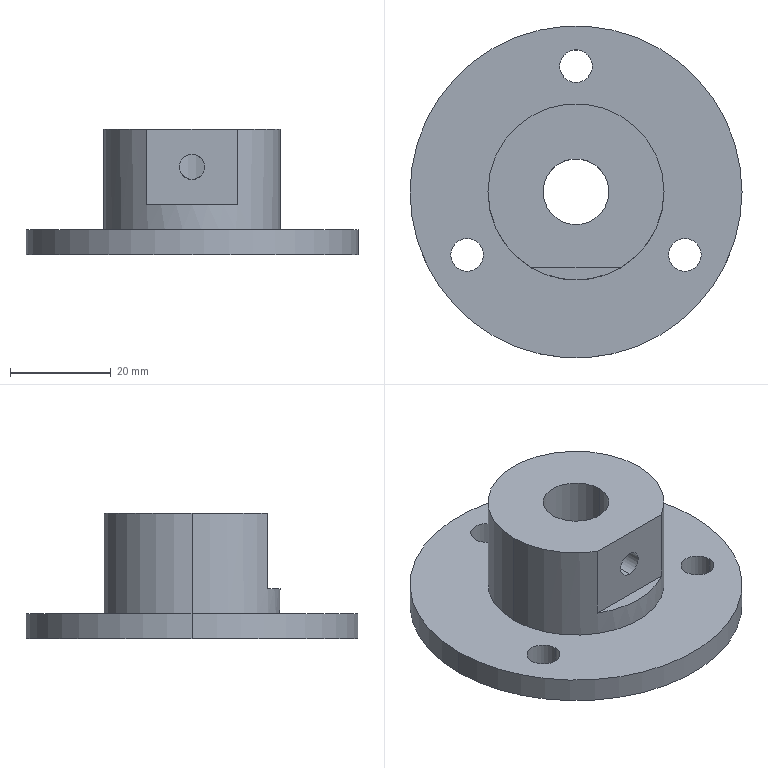Part | STEP file | 11-FG-B05611 | 1 solid | 19 faces | box 66 x 66 x 25 mm | volume 31855 mm3 | cylinder 14 | plane 5 | commonest cylinder face diameters 6.5 x6 5 x2 13.1 x2 35 x2 66 x2
STEP:
#1=CARTESIAN_POINT('',(0.,-6.55,20.));
#2=VERTEX_POINT('',#1);
#3=CARTESIAN_POINT('',(0.,-6.55,15.));
#4=VERTEX_POINT('',#3);
#5=CARTESIAN_POINT('',(0.,-6.55,20.));
#6=CARTESIAN_POINT('',(-0.1643,-6.55,20.));
#7=CARTESIAN_POINT('',(-0.3307,-6.544,19.984));
#8=CARTESIAN_POINT('',(-0.6548,-6.519,19.918));
#9=CARTESIAN_POINT('',(-0.8113,-6.501,19.87));
#10=CARTESIAN_POINT('',(-1.114,-6.456,19.744));
#11=CARTESIAN_POINT('',(-1.259,-6.429,19.666));
#12=CARTESIAN_POINT('',(-1.529,-6.371,19.485));
#13=CARTESIAN_POINT('',(-1.654,-6.339,19.382));
#14=CARTESIAN_POINT('',(-1.885,-6.274,19.151));
#15=CARTESIAN_POINT('',(-1.987,-6.242,19.025));
#16=CARTESIAN_POINT('',(-2.167,-6.182,18.757));
#17=CARTESIAN_POINT('',(-2.245,-6.153,18.611));
#18=CARTESIAN_POINT('',(-2.371,-6.106,18.309));
#19=CARTESIAN_POINT('',(-2.419,-6.087,18.153));
#20=CARTESIAN_POINT('',(-2.483,-6.061,17.831));
#21=CARTESIAN_POINT('',(-2.5,-6.054,17.664));
#22=CARTESIAN_POINT('',(-2.5,-6.054,17.334));
#23=CARTESIAN_POINT('',(-2.484,-6.061,17.17));
#24=CARTESIAN_POINT('',(-2.419,-6.087,16.846));
#25=CARTESIAN_POINT('',(-2.37,-6.107,16.687));
#26=CARTESIAN_POINT('',(-2.244,-6.154,16.386));
#27=CARTESIAN_POINT('',(-2.166,-6.182,16.241));
#28=CARTESIAN_POINT('',(-1.984,-6.243,15.971));
#29=CARTESIAN_POINT('',(-1.882,-6.275,15.846));
#30=CARTESIAN_POINT('',(-1.652,-6.339,15.617));
#31=CARTESIAN_POINT('',(-1.525,-6.371,15.512));
#32=CARTESIAN_POINT('',(-1.256,-6.43,15.332));
#33=CARTESIAN_POINT('',(-1.113,-6.457,15.255));
#34=CARTESIAN_POINT('',(-0.8089,-6.502,15.129));
#35=CARTESIAN_POINT('',(-0.6508,-6.52,15.081));
#36=CARTESIAN_POINT('',(-0.3304,-6.544,15.017));
#37=CARTESIAN_POINT('',(-0.1669,-6.55,15.));
#38=CARTESIAN_POINT('',(0.,-6.55,15.));
#39=B_SPLINE_CURVE_WITH_KNOTS('',3,(#5,#6,#7,#8,#9,#10,#11,#12,#13,#14,#15,#16,#17,#18,#19,#20,#21,#22,#23,#24,#25,#26,#27,#28,#29,#30,#31,#32,#33,#34,#35,#36,#37,#38),.UNSPECIFIED.,.F.,.F.,(4,2,2,2,2,2,2,2,2,2,2,2,2,2,2,2,4),(0.007892,0.008385,0.008878,0.009371,0.009864,0.01036,0.01085,0.01134,0.01184,0.01233,0.01282,0.01332,0.01381,0.0143,0.0148,0.01529,0.01578),.UNSPECIFIED.);
#40=EDGE_CURVE('',#2,#4,#39,.T.);
#41=ORIENTED_EDGE('',*,*,#40,.F.);
#42=CARTESIAN_POINT('',(0.,-15.,20.));
#43=VERTEX_POINT('',#42);
#44=CARTESIAN_POINT('',(0.,-15.,20.));
#45=DIRECTION('',(0.,-1.,0.));
#46=VECTOR('',#45,1000.);
#47=LINE('',#44,#46);
#48=EDGE_CURVE('',#2,#43,#47,.T.);
#49=ORIENTED_EDGE('',*,*,#48,.T.);
#50=CARTESIAN_POINT('',(0.,-15.,15.));
#51=VERTEX_POINT('',#50);
#52=CARTESIAN_POINT('',(0.,-15.,17.5));
#53=DIRECTION('',(0.,-1.,0.));
#54=DIRECTION('',(0.,0.,-1.));
#55=AXIS2_PLACEMENT_3D('',#52,#53,#54);
#56=CIRCLE('',#55,2.5);
#57=EDGE_CURVE('',#43,#51,#56,.T.);
#58=ORIENTED_EDGE('',*,*,#57,.T.);
#59=CARTESIAN_POINT('',(0.,-15.,15.));
#60=DIRECTION('',(0.,-1.,0.));
#61=VECTOR('',#60,1000.);
#62=LINE('',#59,#61);
#63=EDGE_CURVE('',#4,#51,#62,.T.);
#64=ORIENTED_EDGE('',*,*,#63,.F.);
#65=EDGE_LOOP('',(#41,#49,#58,#64));
#66=FACE_OUTER_BOUND('',#65,.T.);
#67=CARTESIAN_POINT('',(0.,-15.,17.5));
#68=DIRECTION('',(0.,-1.,0.));
#69=DIRECTION('',(0.,0.,-1.));
#70=AXIS2_PLACEMENT_3D('',#67,#68,#69);
#71=CYLINDRICAL_SURFACE('',#70,2.5);
#72=ADVANCED_FACE('',(#66),#71,.F.);
#73=CARTESIAN_POINT('',(-24.901,-12.5,0.));
#74=VERTEX_POINT('',#73);
#75=CARTESIAN_POINT('',(-18.401,-12.5,0.));
#76=VERTEX_POINT('',#75);
#77=CARTESIAN_POINT('',(-21.651,-12.5,0.));
#78=DIRECTION('',(0.,0.,1.));
#79=DIRECTION('',(1.,0.,0.));
#80=AXIS2_PLACEMENT_3D('',#77,#78,#79);
#81=CIRCLE('',#80,3.25);
#82=EDGE_CURVE('',#74,#76,#81,.T.);
#83=ORIENTED_EDGE('',*,*,#82,.F.);
#84=CARTESIAN_POINT('',(-24.901,-12.5,5.));
#85=VERTEX_POINT('',#84);
#86=CARTESIAN_POINT('',(-24.901,-12.5,-15.));
#87=DIRECTION('',(0.,0.,1.));
#88=VECTOR('',#87,1000.);
#89=LINE('',#86,#88);
#90=EDGE_CURVE('',#74,#85,#89,.T.);
#91=ORIENTED_EDGE('',*,*,#90,.T.);
#92=CARTESIAN_POINT('',(-18.401,-12.5,5.));
#93=VERTEX_POINT('',#92);
#94=CARTESIAN_POINT('',(-21.651,-12.5,5.));
#95=DIRECTION('',(0.,0.,1.));
#96=DIRECTION('',(-0.5,0.866,0.));
#97=AXIS2_PLACEMENT_3D('',#94,#95,#96);
#98=CIRCLE('',#97,3.25);
#99=EDGE_CURVE('',#85,#93,#98,.T.);
#100=ORIENTED_EDGE('',*,*,#99,.T.);
#101=CARTESIAN_POINT('',(-18.401,-12.5,-15.));
#102=DIRECTION('',(0.,0.,1.));
#103=VECTOR('',#102,1000.);
#104=LINE('',#101,#103);
#105=EDGE_CURVE('',#76,#93,#104,.T.);
#106=ORIENTED_EDGE('',*,*,#105,.F.);
#107=EDGE_LOOP('',(#83,#91,#100,#106));
#108=FACE_OUTER_BOUND('',#107,.T.);
#109=CARTESIAN_POINT('',(-21.651,-12.5,-15.));
#110=DIRECTION('',(0.,0.,1.));
#111=DIRECTION('',(1.,0.,0.));
#112=AXIS2_PLACEMENT_3D('',#109,#110,#111);
#113=CYLINDRICAL_SURFACE('',#112,3.25);
#114=ADVANCED_FACE('',(#108),#113,.F.);
#115=CARTESIAN_POINT('',(18.401,-12.5,0.));
#116=VERTEX_POINT('',#115);
#117=CARTESIAN_POINT('',(24.901,-12.5,0.));
#118=VERTEX_POINT('',#117);
#119=CARTESIAN_POINT('',(21.651,-12.5,0.));
#120=DIRECTION('',(0.,0.,1.));
#121=DIRECTION('',(1.,0.,0.));
#122=AXIS2_PLACEMENT_3D('',#119,#120,#121);
#123=CIRCLE('',#122,3.25);
#124=EDGE_CURVE('',#116,#118,#123,.T.);
#125=ORIENTED_EDGE('',*,*,#124,.F.);
#126=CARTESIAN_POINT('',(18.401,-12.5,5.));
#127=VERTEX_POINT('',#126);
#128=CARTESIAN_POINT('',(18.401,-12.5,-15.));
#129=DIRECTION('',(0.,0.,1.));
#130=VECTOR('',#129,1000.);
#131=LINE('',#128,#130);
#132=EDGE_CURVE('',#116,#127,#131,.T.);
#133=ORIENTED_EDGE('',*,*,#132,.T.);
#134=CARTESIAN_POINT('',(24.901,-12.5,5.));
#135=VERTEX_POINT('',#134);
#136=CARTESIAN_POINT('',(21.651,-12.5,5.));
#137=DIRECTION('',(0.,0.,1.));
#138=DIRECTION('',(-0.5,-0.866,0.));
#139=AXIS2_PLACEMENT_3D('',#136,#137,#138);
#140=CIRCLE('',#139,3.25);
#141=EDGE_CURVE('',#127,#135,#140,.T.);
#142=ORIENTED_EDGE('',*,*,#141,.T.);
#143=CARTESIAN_POINT('',(24.901,-12.5,-15.));
#144=DIRECTION('',(0.,0.,1.));
#145=VECTOR('',#144,1000.);
#146=LINE('',#143,#145);
#147=EDGE_CURVE('',#118,#135,#146,.T.);
#148=ORIENTED_EDGE('',*,*,#147,.F.);
#149=EDGE_LOOP('',(#125,#133,#142,#148));
#150=FACE_OUTER_BOUND('',#149,.T.);
#151=CARTESIAN_POINT('',(21.651,-12.5,-15.));
#152=DIRECTION('',(0.,0.,1.));
#153=DIRECTION('',(1.,0.,0.));
#154=AXIS2_PLACEMENT_3D('',#151,#152,#153);
#155=CYLINDRICAL_SURFACE('',#154,3.25);
#156=ADVANCED_FACE('',(#150),#155,.F.);
#157=CARTESIAN_POINT('',(-3.25,25.,0.));
#158=VERTEX_POINT('',#157);
#159=CARTESIAN_POINT('',(3.25,25.,0.));
#160=VERTEX_POINT('',#159);
#161=CARTESIAN_POINT('',(0.,25.,0.));
#162=DIRECTION('',(0.,0.,1.));
#163=DIRECTION('',(1.,0.,0.));
#164=AXIS2_PLACEMENT_3D('',#161,#162,#163);
#165=CIRCLE('',#164,3.25);
#166=EDGE_CURVE('',#158,#160,#165,.T.);
#167=ORIENTED_EDGE('',*,*,#166,.F.);
#168=CARTESIAN_POINT('',(-3.25,25.,5.));
#169=VERTEX_POINT('',#168);
#170=CARTESIAN_POINT('',(-3.25,25.,-15.));
#171=DIRECTION('',(0.,0.,1.));
#172=VECTOR('',#171,1000.);
#173=LINE('',#170,#172);
#174=EDGE_CURVE('',#158,#169,#173,.T.);
#175=ORIENTED_EDGE('',*,*,#174,.T.);
#176=CARTESIAN_POINT('',(3.25,25.,5.));
#177=VERTEX_POINT('',#176);
#178=CARTESIAN_POINT('',(0.,25.,5.));
#179=DIRECTION('',(0.,0.,1.));
#180=DIRECTION('',(1.,0.,0.));
#181=AXIS2_PLACEMENT_3D('',#178,#179,#180);
#182=CIRCLE('',#181,3.25);
#183=EDGE_CURVE('',#169,#177,#182,.T.);
#184=ORIENTED_EDGE('',*,*,#183,.T.);
#185=CARTESIAN_POINT('',(3.25,25.,-15.));
#186=DIRECTION('',(0.,0.,1.));
#187=VECTOR('',#186,1000.);
#188=LINE('',#185,#187);
#189=EDGE_CURVE('',#160,#177,#188,.T.);
#190=ORIENTED_EDGE('',*,*,#189,.F.);
#191=EDGE_LOOP('',(#167,#175,#184,#190));
#192=FACE_OUTER_BOUND('',#191,.T.);
#193=CARTESIAN_POINT('',(0.,25.,-15.));
#194=DIRECTION('',(0.,0.,1.));
#195=DIRECTION('',(1.,0.,0.));
#196=AXIS2_PLACEMENT_3D('',#193,#194,#195);
#197=CYLINDRICAL_SURFACE('',#196,3.25);
#198=ADVANCED_FACE('',(#192),#197,.F.);
#199=CARTESIAN_POINT('',(0.,-6.55,15.));
#200=CARTESIAN_POINT('',(0.1669,-6.55,15.));
#201=CARTESIAN_POINT('',(0.3307,-6.544,15.017));
#202=CARTESIAN_POINT('',(0.6525,-6.519,15.081));
#203=CARTESIAN_POINT('',(0.8121,-6.501,15.13));
#204=CARTESIAN_POINT('',(1.114,-6.456,15.256));
#205=CARTESIAN_POINT('',(1.257,-6.43,15.333));
#206=CARTESIAN_POINT('',(1.528,-6.371,15.515));
#207=CARTESIAN_POINT('',(1.655,-6.339,15.619));
#208=CARTESIAN_POINT('',(1.997,-6.243,15.962));
#209=CARTESIAN_POINT('',(2.182,-6.177,16.238));
#210=CARTESIAN_POINT('',(2.37,-6.107,16.688));
#211=CARTESIAN_POINT('',(2.419,-6.087,16.847));
#212=CARTESIAN_POINT('',(2.484,-6.061,17.17));
#213=CARTESIAN_POINT('',(2.5,-6.054,17.334));
#214=CARTESIAN_POINT('',(2.5,-6.054,17.663));
#215=CARTESIAN_POINT('',(2.483,-6.061,17.831));
#216=CARTESIAN_POINT('',(2.419,-6.087,18.153));
#217=CARTESIAN_POINT('',(2.371,-6.106,18.31));
#218=CARTESIAN_POINT('',(2.244,-6.154,18.614));
#219=CARTESIAN_POINT('',(2.167,-6.182,18.758));
#220=CARTESIAN_POINT('',(1.986,-6.242,19.027));
#221=CARTESIAN_POINT('',(1.882,-6.275,19.154));
#222=CARTESIAN_POINT('',(1.652,-6.339,19.383));
#223=CARTESIAN_POINT('',(1.528,-6.371,19.486));
#224=CARTESIAN_POINT('',(1.258,-6.43,19.667));
#225=CARTESIAN_POINT('',(1.112,-6.457,19.745));
#226=CARTESIAN_POINT('',(0.811,-6.501,19.87));
#227=CARTESIAN_POINT('',(0.6548,-6.519,19.918));
#228=CARTESIAN_POINT('',(0.3297,-6.544,19.984));
#229=CARTESIAN_POINT('',(0.1644,-6.55,20.));
#230=CARTESIAN_POINT('',(0.,-6.55,20.));
#231=B_SPLINE_CURVE_WITH_KNOTS('',3,(#199,#200,#201,#202,#203,#204,#205,#206,#207,#208,#209,#210,#211,#212,#213,#214,#215,#216,#217,#218,#219,#220,#221,#222,#223,#224,#225,#226,#227,#228,#229,#230),.UNSPECIFIED.,.F.,.F.,(4,2,2,2,2,2,2,2,2,2,2,2,2,2,2,4),(0.,0.0004932,0.0009865,0.00148,0.001973,0.002959,0.003453,0.003946,0.004439,0.004932,0.005426,0.005919,0.006412,0.006905,0.007399,0.007892),.UNSPECIFIED.);
#232=EDGE_CURVE('',#4,#2,#231,.T.);
#233=ORIENTED_EDGE('',*,*,#232,.T.);
#234=ORIENTED_EDGE('',*,*,#40,.T.);
#235=EDGE_LOOP('',(#233,#234));
#236=FACE_BOUND('',#235,.T.);
#237=CARTESIAN_POINT('',(-6.55,0.,0.));
#238=VERTEX_POINT('',#237);
#239=CARTESIAN_POINT('',(6.55,0.,0.));
#240=VERTEX_POINT('',#239);
#241=CARTESIAN_POINT('',(0.,0.,0.));
#242=DIRECTION('',(0.,0.,1.));
#243=DIRECTION('',(1.,0.,0.));
#244=AXIS2_PLACEMENT_3D('',#241,#242,#243);
#245=CIRCLE('',#244,6.55);
#246=EDGE_CURVE('',#238,#240,#245,.T.);
#247=ORIENTED_EDGE('',*,*,#246,.F.);
#248=CARTESIAN_POINT('',(-6.55,0.,25.));
#249=VERTEX_POINT('',#248);
#250=CARTESIAN_POINT('',(-6.55,0.,0.));
#251=DIRECTION('',(0.,0.,1.));
#252=VECTOR('',#251,1000.);
#253=LINE('',#250,#252);
#254=EDGE_CURVE('',#238,#249,#253,.T.);
#255=ORIENTED_EDGE('',*,*,#254,.T.);
#256=CARTESIAN_POINT('',(6.55,0.,25.));
#257=VERTEX_POINT('',#256);
#258=CARTESIAN_POINT('',(0.,0.,25.));
#259=DIRECTION('',(0.,0.,1.));
#260=DIRECTION('',(1.,0.,0.));
#261=AXIS2_PLACEMENT_3D('',#258,#259,#260);
#262=CIRCLE('',#261,6.55);
#263=EDGE_CURVE('',#249,#257,#262,.T.);
#264=ORIENTED_EDGE('',*,*,#263,.T.);
#265=CARTESIAN_POINT('',(6.55,0.,0.));
#266=DIRECTION('',(0.,0.,1.));
#267=VECTOR('',#266,1000.);
#268=LINE('',#265,#267);
#269=EDGE_CURVE('',#240,#257,#268,.T.);
#270=ORIENTED_EDGE('',*,*,#269,.F.);
#271=EDGE_LOOP('',(#247,#255,#264,#270));
#272=FACE_OUTER_BOUND('',#271,.T.);
#273=CARTESIAN_POINT('',(0.,0.,0.));
#274=DIRECTION('',(0.,0.,1.));
#275=DIRECTION('',(1.,0.,0.));
#276=AXIS2_PLACEMENT_3D('',#273,#274,#275);
#277=CYLINDRICAL_SURFACE('',#276,6.55);
#278=ADVANCED_FACE('',(#236,#272),#277,.F.);
#279=CARTESIAN_POINT('',(17.5,0.,25.));
#280=VERTEX_POINT('',#279);
#281=CARTESIAN_POINT('',(-17.5,0.,25.));
#282=VERTEX_POINT('',#281);
#283=CARTESIAN_POINT('',(0.,0.,25.));
#284=DIRECTION('',(0.,0.,1.));
#285=DIRECTION('',(1.,0.,0.));
#286=AXIS2_PLACEMENT_3D('',#283,#284,#285);
#287=CIRCLE('',#286,17.5);
#288=EDGE_CURVE('',#280,#282,#287,.T.);
#289=ORIENTED_EDGE('',*,*,#288,.F.);
#290=CARTESIAN_POINT('',(17.5,0.,5.));
#291=VERTEX_POINT('',#290);
#292=CARTESIAN_POINT('',(17.5,0.,25.));
#293=DIRECTION('',(0.,0.,-1.));
#294=VECTOR('',#293,1000.);
#295=LINE('',#292,#294);
#296=EDGE_CURVE('',#280,#291,#295,.T.);
#297=ORIENTED_EDGE('',*,*,#296,.T.);
#298=CARTESIAN_POINT('',(-17.5,0.,5.));
#299=VERTEX_POINT('',#298);
#300=CARTESIAN_POINT('',(0.,0.,5.));
#301=DIRECTION('',(0.,0.,1.));
#302=DIRECTION('',(1.,0.,0.));
#303=AXIS2_PLACEMENT_3D('',#300,#301,#302);
#304=CIRCLE('',#303,17.5);
#305=EDGE_CURVE('',#291,#299,#304,.T.);
#306=ORIENTED_EDGE('',*,*,#305,.T.);
#307=CARTESIAN_POINT('',(-17.5,0.,25.));
#308=DIRECTION('',(0.,0.,-1.));
#309=VECTOR('',#308,1000.);
#310=LINE('',#307,#309);
#311=EDGE_CURVE('',#282,#299,#310,.T.);
#312=ORIENTED_EDGE('',*,*,#311,.F.);
#313=EDGE_LOOP('',(#289,#297,#306,#312));
#314=FACE_OUTER_BOUND('',#313,.T.);
#315=CARTESIAN_POINT('',(0.,0.,25.));
#316=DIRECTION('',(0.,0.,-1.));
#317=DIRECTION('',(-1.,0.,0.));
#318=AXIS2_PLACEMENT_3D('',#315,#316,#317);
#319=CYLINDRICAL_SURFACE('',#318,17.5);
#320=ADVANCED_FACE('',(#314),#319,.T.);
#321=CARTESIAN_POINT('',(33.,0.,5.));
#322=VERTEX_POINT('',#321);
#323=CARTESIAN_POINT('',(-33.,0.,5.));
#324=VERTEX_POINT('',#323);
#325=CARTESIAN_POINT('',(0.,0.,5.));
#326=DIRECTION('',(0.,0.,1.));
#327=DIRECTION('',(1.,0.,0.));
#328=AXIS2_PLACEMENT_3D('',#325,#326,#327);
#329=CIRCLE('',#328,33.);
#330=EDGE_CURVE('',#322,#324,#329,.T.);
#331=ORIENTED_EDGE('',*,*,#330,.F.);
#332=CARTESIAN_POINT('',(33.,0.,0.));
#333=VERTEX_POINT('',#332);
#334=CARTESIAN_POINT('',(33.,0.,5.));
#335=DIRECTION('',(0.,0.,-1.));
#336=VECTOR('',#335,1000.);
#337=LINE('',#334,#336);
#338=EDGE_CURVE('',#322,#333,#337,.T.);
#339=ORIENTED_EDGE('',*,*,#338,.T.);
#340=CARTESIAN_POINT('',(-33.,0.,0.));
#341=VERTEX_POINT('',#340);
#342=CARTESIAN_POINT('',(0.,0.,0.));
#343=DIRECTION('',(0.,0.,1.));
#344=DIRECTION('',(1.,0.,0.));
#345=AXIS2_PLACEMENT_3D('',#342,#343,#344);
#346=CIRCLE('',#345,33.);
#347=EDGE_CURVE('',#333,#341,#346,.T.);
#348=ORIENTED_EDGE('',*,*,#347,.T.);
#349=CARTESIAN_POINT('',(-33.,0.,5.));
#350=DIRECTION('',(0.,0.,-1.));
#351=VECTOR('',#350,1000.);
#352=LINE('',#349,#351);
#353=EDGE_CURVE('',#324,#341,#352,.T.);
#354=ORIENTED_EDGE('',*,*,#353,.F.);
#355=EDGE_LOOP('',(#331,#339,#348,#354));
#356=FACE_OUTER_BOUND('',#355,.T.);
#357=CARTESIAN_POINT('',(0.,0.,5.));
#358=DIRECTION('',(0.,0.,-1.));
#359=DIRECTION('',(-1.,0.,0.));
#360=AXIS2_PLACEMENT_3D('',#357,#358,#359);
#361=CYLINDRICAL_SURFACE('',#360,33.);
#362=ADVANCED_FACE('',(#356),#361,.T.);
#363=CARTESIAN_POINT('',(-21.651,-12.5,5.));
#364=DIRECTION('',(0.,0.,1.));
#365=DIRECTION('',(-0.5,0.866,0.));
#366=AXIS2_PLACEMENT_3D('',#363,#364,#365);
#367=CIRCLE('',#366,3.25);
#368=EDGE_CURVE('',#93,#85,#367,.T.);
#369=ORIENTED_EDGE('',*,*,#368,.F.);
#370=ORIENTED_EDGE('',*,*,#99,.F.);
#371=EDGE_LOOP('',(#369,#370));
#372=FACE_BOUND('',#371,.T.);
#373=CARTESIAN_POINT('',(21.651,-12.5,5.));
#374=DIRECTION('',(0.,0.,1.));
#375=DIRECTION('',(-0.5,-0.866,0.));
#376=AXIS2_PLACEMENT_3D('',#373,#374,#375);
#377=CIRCLE('',#376,3.25);
#378=EDGE_CURVE('',#135,#127,#377,.T.);
#379=ORIENTED_EDGE('',*,*,#378,.F.);
#380=ORIENTED_EDGE('',*,*,#141,.F.);
#381=EDGE_LOOP('',(#379,#380));
#382=FACE_BOUND('',#381,.T.);
#383=CARTESIAN_POINT('',(0.,25.,5.));
#384=DIRECTION('',(0.,0.,1.));
#385=DIRECTION('',(1.,0.,0.));
#386=AXIS2_PLACEMENT_3D('',#383,#384,#385);
#387=CIRCLE('',#386,3.25);
#388=EDGE_CURVE('',#177,#169,#387,.T.);
#389=ORIENTED_EDGE('',*,*,#388,.F.);
#390=ORIENTED_EDGE('',*,*,#183,.F.);
#391=EDGE_LOOP('',(#389,#390));
#392=FACE_BOUND('',#391,.T.);
#393=CARTESIAN_POINT('',(0.,0.,5.));
#394=DIRECTION('',(0.,0.,1.));
#395=DIRECTION('',(1.,0.,0.));
#396=AXIS2_PLACEMENT_3D('',#393,#394,#395);
#397=CIRCLE('',#396,33.);
#398=EDGE_CURVE('',#324,#322,#397,.T.);
#399=ORIENTED_EDGE('',*,*,#398,.T.);
#400=ORIENTED_EDGE('',*,*,#330,.T.);
#401=EDGE_LOOP('',(#399,#400));
#402=FACE_OUTER_BOUND('',#401,.T.);
#403=CARTESIAN_POINT('',(0.,0.,5.));
#404=DIRECTION('',(0.,0.,1.));
#405=DIRECTION('',(1.,0.,0.));
#406=AXIS2_PLACEMENT_3D('',#403,#404,#405);
#407=CIRCLE('',#406,17.5);
#408=EDGE_CURVE('',#299,#291,#407,.T.);
#409=ORIENTED_EDGE('',*,*,#408,.F.);
#410=ORIENTED_EDGE('',*,*,#305,.F.);
#411=EDGE_LOOP('',(#409,#410));
#412=FACE_BOUND('',#411,.T.);
#413=CARTESIAN_POINT('',(0.,0.,5.));
#414=DIRECTION('',(0.,0.,1.));
#415=DIRECTION('',(1.,0.,0.));
#416=AXIS2_PLACEMENT_3D('',#413,#414,#415);
#417=PLANE('',#416);
#418=ADVANCED_FACE('',(#372,#382,#392,#402,#412),#417,.T.);
#419=ORIENTED_EDGE('',*,*,#338,.F.);
#420=ORIENTED_EDGE('',*,*,#398,.F.);
#421=ORIENTED_EDGE('',*,*,#353,.T.);
#422=CARTESIAN_POINT('',(0.,0.,0.));
#423=DIRECTION('',(0.,0.,1.));
#424=DIRECTION('',(1.,0.,0.));
#425=AXIS2_PLACEMENT_3D('',#422,#423,#424);
#426=CIRCLE('',#425,33.);
#427=EDGE_CURVE('',#341,#333,#426,.T.);
#428=ORIENTED_EDGE('',*,*,#427,.T.);
#429=EDGE_LOOP('',(#419,#420,#421,#428));
#430=FACE_OUTER_BOUND('',#429,.T.);
#431=CARTESIAN_POINT('',(0.,0.,5.));
#432=DIRECTION('',(0.,0.,-1.));
#433=DIRECTION('',(-1.,0.,0.));
#434=AXIS2_PLACEMENT_3D('',#431,#432,#433);
#435=CYLINDRICAL_SURFACE('',#434,33.);
#436=ADVANCED_FACE('',(#430),#435,.T.);
#437=CARTESIAN_POINT('',(-21.651,-12.5,0.));
#438=DIRECTION('',(0.,0.,1.));
#439=DIRECTION('',(1.,0.,0.));
#440=AXIS2_PLACEMENT_3D('',#437,#438,#439);
#441=CIRCLE('',#440,3.25);
#442=EDGE_CURVE('',#76,#74,#441,.T.);
#443=ORIENTED_EDGE('',*,*,#442,.T.);
#444=ORIENTED_EDGE('',*,*,#82,.T.);
#445=EDGE_LOOP('',(#443,#444));
#446=FACE_BOUND('',#445,.T.);
#447=CARTESIAN_POINT('',(21.651,-12.5,0.));
#448=DIRECTION('',(0.,0.,1.));
#449=DIRECTION('',(1.,0.,0.));
#450=AXIS2_PLACEMENT_3D('',#447,#448,#449);
#451=CIRCLE('',#450,3.25);
#452=EDGE_CURVE('',#118,#116,#451,.T.);
#453=ORIENTED_EDGE('',*,*,#452,.T.);
#454=ORIENTED_EDGE('',*,*,#124,.T.);
#455=EDGE_LOOP('',(#453,#454));
#456=FACE_BOUND('',#455,.T.);
#457=CARTESIAN_POINT('',(0.,25.,0.));
#458=DIRECTION('',(0.,0.,1.));
#459=DIRECTION('',(1.,0.,0.));
#460=AXIS2_PLACEMENT_3D('',#457,#458,#459);
#461=CIRCLE('',#460,3.25);
#462=EDGE_CURVE('',#160,#158,#461,.T.);
#463=ORIENTED_EDGE('',*,*,#462,.T.);
#464=ORIENTED_EDGE('',*,*,#166,.T.);
#465=EDGE_LOOP('',(#463,#464));
#466=FACE_BOUND('',#465,.T.);
#467=CARTESIAN_POINT('',(0.,0.,0.));
#468=DIRECTION('',(0.,0.,1.));
#469=DIRECTION('',(1.,0.,0.));
#470=AXIS2_PLACEMENT_3D('',#467,#468,#469);
#471=CIRCLE('',#470,6.55);
#472=EDGE_CURVE('',#240,#238,#471,.T.);
#473=ORIENTED_EDGE('',*,*,#472,.T.);
#474=ORIENTED_EDGE('',*,*,#246,.T.);
#475=EDGE_LOOP('',(#473,#474));
#476=FACE_BOUND('',#475,.T.);
#477=ORIENTED_EDGE('',*,*,#427,.F.);
#478=ORIENTED_EDGE('',*,*,#347,.F.);
#479=EDGE_LOOP('',(#477,#478));
#480=FACE_OUTER_BOUND('',#479,.T.);
#481=CARTESIAN_POINT('',(0.,0.,0.));
#482=DIRECTION('',(0.,0.,1.));
#483=DIRECTION('',(1.,0.,0.));
#484=AXIS2_PLACEMENT_3D('',#481,#482,#483);
#485=PLANE('',#484);
#486=ADVANCED_FACE('',(#446,#456,#466,#476,#480),#485,.F.);
#487=ORIENTED_EDGE('',*,*,#296,.F.);
#488=CARTESIAN_POINT('',(9.014,-15.,25.));
#489=VERTEX_POINT('',#488);
#490=CARTESIAN_POINT('',(0.,0.,25.));
#491=DIRECTION('',(0.,0.,1.));
#492=DIRECTION('',(1.,0.,0.));
#493=AXIS2_PLACEMENT_3D('',#490,#491,#492);
#494=CIRCLE('',#493,17.5);
#495=EDGE_CURVE('',#489,#280,#494,.T.);
#496=ORIENTED_EDGE('',*,*,#495,.F.);
#497=CARTESIAN_POINT('',(9.014,-15.,10.));
#498=VERTEX_POINT('',#497);
#499=CARTESIAN_POINT('',(9.014,-15.,25.));
#500=DIRECTION('',(0.,0.,-1.));
#501=VECTOR('',#500,1000.);
#502=LINE('',#499,#501);
#503=EDGE_CURVE('',#489,#498,#502,.T.);
#504=ORIENTED_EDGE('',*,*,#503,.T.);
#505=CARTESIAN_POINT('',(-9.014,-15.,10.));
#506=VERTEX_POINT('',#505);
#507=CARTESIAN_POINT('',(0.,0.,10.));
#508=DIRECTION('',(0.,0.,1.));
#509=DIRECTION('',(1.,0.,0.));
#510=AXIS2_PLACEMENT_3D('',#507,#508,#509);
#511=CIRCLE('',#510,17.5);
#512=EDGE_CURVE('',#506,#498,#511,.T.);
#513=ORIENTED_EDGE('',*,*,#512,.F.);
#514=CARTESIAN_POINT('',(-9.014,-15.,25.));
#515=VERTEX_POINT('',#514);
#516=CARTESIAN_POINT('',(-9.014,-15.,25.));
#517=DIRECTION('',(0.,0.,1.));
#518=VECTOR('',#517,1000.);
#519=LINE('',#516,#518);
#520=EDGE_CURVE('',#506,#515,#519,.T.);
#521=ORIENTED_EDGE('',*,*,#520,.T.);
#522=CARTESIAN_POINT('',(0.,0.,25.));
#523=DIRECTION('',(0.,0.,1.));
#524=DIRECTION('',(1.,0.,0.));
#525=AXIS2_PLACEMENT_3D('',#522,#523,#524);
#526=CIRCLE('',#525,17.5);
#527=EDGE_CURVE('',#282,#515,#526,.T.);
#528=ORIENTED_EDGE('',*,*,#527,.F.);
#529=ORIENTED_EDGE('',*,*,#311,.T.);
#530=ORIENTED_EDGE('',*,*,#408,.T.);
#531=EDGE_LOOP('',(#487,#496,#504,#513,#521,#528,#529,#530));
#532=FACE_OUTER_BOUND('',#531,.T.);
#533=CARTESIAN_POINT('',(0.,0.,25.));
#534=DIRECTION('',(0.,0.,-1.));
#535=DIRECTION('',(-1.,0.,0.));
#536=AXIS2_PLACEMENT_3D('',#533,#534,#535);
#537=CYLINDRICAL_SURFACE('',#536,17.5);
#538=ADVANCED_FACE('',(#532),#537,.T.);
#539=CARTESIAN_POINT('',(0.,-15.,25.));
#540=DIRECTION('',(-1.,0.,0.));
#541=VECTOR('',#540,1000.);
#542=LINE('',#539,#541);
#543=EDGE_CURVE('',#489,#515,#542,.T.);
#544=ORIENTED_EDGE('',*,*,#543,.F.);
#545=ORIENTED_EDGE('',*,*,#495,.T.);
#546=ORIENTED_EDGE('',*,*,#288,.T.);
#547=ORIENTED_EDGE('',*,*,#527,.T.);
#548=EDGE_LOOP('',(#544,#545,#546,#547));
#549=FACE_OUTER_BOUND('',#548,.T.);
#550=CARTESIAN_POINT('',(0.,0.,25.));
#551=DIRECTION('',(0.,0.,1.));
#552=DIRECTION('',(1.,0.,0.));
#553=AXIS2_PLACEMENT_3D('',#550,#551,#552);
#554=CIRCLE('',#553,6.55);
#555=EDGE_CURVE('',#257,#249,#554,.T.);
#556=ORIENTED_EDGE('',*,*,#555,.F.);
#557=ORIENTED_EDGE('',*,*,#263,.F.);
#558=EDGE_LOOP('',(#556,#557));
#559=FACE_BOUND('',#558,.T.);
#560=CARTESIAN_POINT('',(0.,0.,25.));
#561=DIRECTION('',(0.,0.,1.));
#562=DIRECTION('',(1.,0.,0.));
#563=AXIS2_PLACEMENT_3D('',#560,#561,#562);
#564=PLANE('',#563);
#565=ADVANCED_FACE('',(#549,#559),#564,.T.);
#566=ORIENTED_EDGE('',*,*,#254,.F.);
#567=ORIENTED_EDGE('',*,*,#472,.F.);
#568=ORIENTED_EDGE('',*,*,#269,.T.);
#569=ORIENTED_EDGE('',*,*,#555,.T.);
#570=EDGE_LOOP('',(#566,#567,#568,#569));
#571=FACE_OUTER_BOUND('',#570,.T.);
#572=CARTESIAN_POINT('',(0.,0.,0.));
#573=DIRECTION('',(0.,0.,1.));
#574=DIRECTION('',(1.,0.,0.));
#575=AXIS2_PLACEMENT_3D('',#572,#573,#574);
#576=CYLINDRICAL_SURFACE('',#575,6.55);
#577=ADVANCED_FACE('',(#571),#576,.F.);
#578=ORIENTED_EDGE('',*,*,#174,.F.);
#579=ORIENTED_EDGE('',*,*,#462,.F.);
#580=ORIENTED_EDGE('',*,*,#189,.T.);
#581=ORIENTED_EDGE('',*,*,#388,.T.);
#582=EDGE_LOOP('',(#578,#579,#580,#581));
#583=FACE_OUTER_BOUND('',#582,.T.);
#584=CARTESIAN_POINT('',(0.,25.,-15.));
#585=DIRECTION('',(0.,0.,1.));
#586=DIRECTION('',(1.,0.,0.));
#587=AXIS2_PLACEMENT_3D('',#584,#585,#586);
#588=CYLINDRICAL_SURFACE('',#587,3.25);
#589=ADVANCED_FACE('',(#583),#588,.F.);
#590=ORIENTED_EDGE('',*,*,#132,.F.);
#591=ORIENTED_EDGE('',*,*,#452,.F.);
#592=ORIENTED_EDGE('',*,*,#147,.T.);
#593=ORIENTED_EDGE('',*,*,#378,.T.);
#594=EDGE_LOOP('',(#590,#591,#592,#593));
#595=FACE_OUTER_BOUND('',#594,.T.);
#596=CARTESIAN_POINT('',(21.651,-12.5,-15.));
#597=DIRECTION('',(0.,0.,1.));
#598=DIRECTION('',(1.,0.,0.));
#599=AXIS2_PLACEMENT_3D('',#596,#597,#598);
#600=CYLINDRICAL_SURFACE('',#599,3.25);
#601=ADVANCED_FACE('',(#595),#600,.F.);
#602=ORIENTED_EDGE('',*,*,#90,.F.);
#603=ORIENTED_EDGE('',*,*,#442,.F.);
#604=ORIENTED_EDGE('',*,*,#105,.T.);
#605=ORIENTED_EDGE('',*,*,#368,.T.);
#606=EDGE_LOOP('',(#602,#603,#604,#605));
#607=FACE_OUTER_BOUND('',#606,.T.);
#608=CARTESIAN_POINT('',(-21.651,-12.5,-15.));
#609=DIRECTION('',(0.,0.,1.));
#610=DIRECTION('',(1.,0.,0.));
#611=AXIS2_PLACEMENT_3D('',#608,#609,#610);
#612=CYLINDRICAL_SURFACE('',#611,3.25);
#613=ADVANCED_FACE('',(#607),#612,.F.);
#614=ORIENTED_EDGE('',*,*,#512,.T.);
#615=CARTESIAN_POINT('',(-44.663,-15.,10.));
#616=DIRECTION('',(-1.,0.,0.));
#617=VECTOR('',#616,1000.);
#618=LINE('',#615,#617);
#619=EDGE_CURVE('',#498,#506,#618,.T.);
#620=ORIENTED_EDGE('',*,*,#619,.T.);
#621=EDGE_LOOP('',(#614,#620));
#622=FACE_OUTER_BOUND('',#621,.T.);
#623=CARTESIAN_POINT('',(-44.663,-46.418,10.));
#624=DIRECTION('',(0.,0.,1.));
#625=DIRECTION('',(1.,0.,0.));
#626=AXIS2_PLACEMENT_3D('',#623,#624,#625);
#627=PLANE('',#626);
#628=ADVANCED_FACE('',(#622),#627,.T.);
#629=CARTESIAN_POINT('',(0.,-15.,17.5));
#630=DIRECTION('',(0.,-1.,0.));
#631=DIRECTION('',(0.,0.,-1.));
#632=AXIS2_PLACEMENT_3D('',#629,#630,#631);
#633=CIRCLE('',#632,2.5);
#634=EDGE_CURVE('',#51,#43,#633,.T.);
#635=ORIENTED_EDGE('',*,*,#634,.F.);
#636=ORIENTED_EDGE('',*,*,#57,.F.);
#637=EDGE_LOOP('',(#635,#636));
#638=FACE_BOUND('',#637,.T.);
#639=ORIENTED_EDGE('',*,*,#543,.T.);
#640=ORIENTED_EDGE('',*,*,#520,.F.);
#641=ORIENTED_EDGE('',*,*,#619,.F.);
#642=ORIENTED_EDGE('',*,*,#503,.F.);
#643=EDGE_LOOP('',(#639,#640,#641,#642));
#644=FACE_OUTER_BOUND('',#643,.T.);
#645=CARTESIAN_POINT('',(-44.663,-15.,10.));
#646=DIRECTION('',(0.,1.,0.));
#647=DIRECTION('',(0.,0.,1.));
#648=AXIS2_PLACEMENT_3D('',#645,#646,#647);
#649=PLANE('',#648);
#650=ADVANCED_FACE('',(#638,#644),#649,.F.);
#651=ORIENTED_EDGE('',*,*,#48,.F.);
#652=ORIENTED_EDGE('',*,*,#232,.F.);
#653=ORIENTED_EDGE('',*,*,#63,.T.);
#654=ORIENTED_EDGE('',*,*,#634,.T.);
#655=EDGE_LOOP('',(#651,#652,#653,#654));
#656=FACE_OUTER_BOUND('',#655,.T.);
#657=CARTESIAN_POINT('',(0.,-15.,17.5));
#658=DIRECTION('',(0.,-1.,0.));
#659=DIRECTION('',(0.,0.,-1.));
#660=AXIS2_PLACEMENT_3D('',#657,#658,#659);
#661=CYLINDRICAL_SURFACE('',#660,2.5);
#662=ADVANCED_FACE('',(#656),#661,.F.);
#663=CLOSED_SHELL('',(#72,#114,#156,#198,#278,#320,#362,#418,#436,#486,#538,#565,#577,#589,#601,#613,#628,#650,#662));
#664=MANIFOLD_SOLID_BREP('',#663);
#665=CARTESIAN_POINT('',(0.,0.,0.));
#666=DIRECTION('',(0.,0.,1.));
#667=DIRECTION('',(1.,0.,0.));
#668=AXIS2_PLACEMENT_3D('',#665,#666,#667);
#669=(LENGTH_UNIT()NAMED_UNIT(*)SI_UNIT(.MILLI.,.METRE.));
#670=UNCERTAINTY_MEASURE_WITH_UNIT(LENGTH_MEASURE(0.00001),#669,'','');
#671=(NAMED_UNIT(*)PLANE_ANGLE_UNIT()SI_UNIT($,.RADIAN.));
#672=(NAMED_UNIT(*)SI_UNIT($,.STERADIAN.)SOLID_ANGLE_UNIT());
#673=(GEOMETRIC_REPRESENTATION_CONTEXT(3)GLOBAL_UNCERTAINTY_ASSIGNED_CONTEXT((#670))GLOBAL_UNIT_ASSIGNED_CONTEXT((#669,#671,#672))REPRESENTATION_CONTEXT('',''));
#674=ADVANCED_BREP_SHAPE_REPRESENTATION('',(#664,#668),#673);